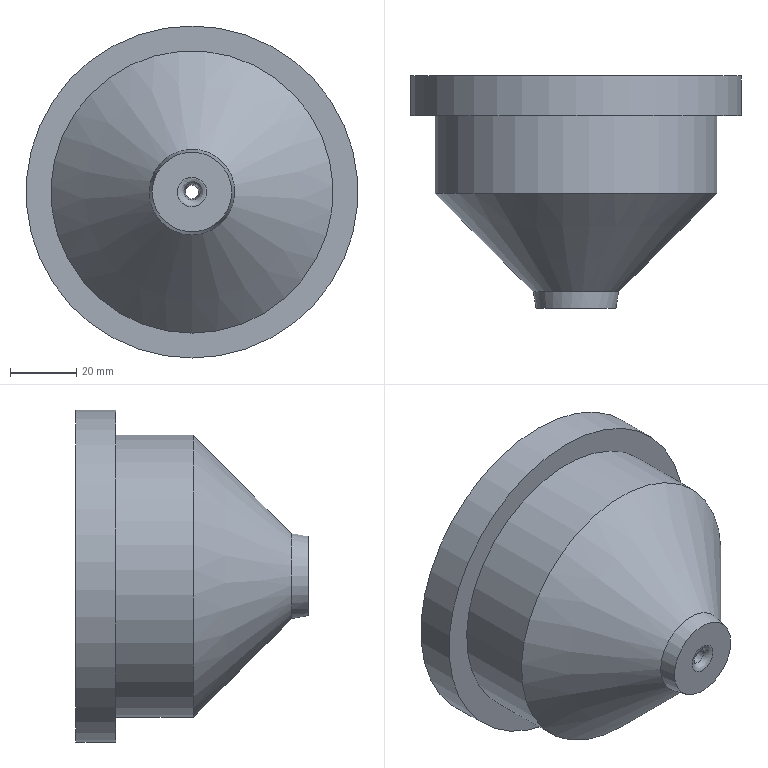Part | STEP file | SPRUE_id462_x_t | 1 solid | 13 faces | box 100 x 70 x 100 mm | volume 170232 mm3 | cone 4 | plane 3 | cylinder 3 | other 2 | spline 1 | commonest cylinder face diameters 65 x1 85 x1 100 x1
STEP:
#1=CARTESIAN_POINT('',(0.,90.5,-4.431));
#2=VERTEX_POINT('',#1);
#3=CARTESIAN_POINT('',(0.,90.5,4.431));
#4=VERTEX_POINT('',#3);
#5=CARTESIAN_POINT('',(0.,90.5,-4.431));
#6=CARTESIAN_POINT('',(0.2789,90.5,-4.431));
#7=CARTESIAN_POINT('',(0.5857,90.5,-4.396));
#8=CARTESIAN_POINT('',(0.906,90.5,-4.341));
#9=CARTESIAN_POINT('',(1.367,90.5,-4.225));
#10=CARTESIAN_POINT('',(1.776,90.5,-4.062));
#11=CARTESIAN_POINT('',(1.91,90.5,-4.001));
#12=CARTESIAN_POINT('',(2.106,90.5,-3.899));
#13=CARTESIAN_POINT('',(2.196,90.5,-3.848));
#14=CARTESIAN_POINT('',(2.22,90.5,-3.835));
#15=CARTESIAN_POINT('',(2.24,90.5,-3.823));
#16=CARTESIAN_POINT('',(2.373,90.5,-3.744));
#17=CARTESIAN_POINT('',(2.599,90.5,-3.611));
#18=CARTESIAN_POINT('',(3.199,90.5,-3.091));
#19=CARTESIAN_POINT('',(3.611,90.5,-2.603));
#20=CARTESIAN_POINT('',(4.042,90.5,-1.864));
#21=CARTESIAN_POINT('',(4.124,90.5,-1.623));
#22=CARTESIAN_POINT('',(4.164,90.5,-1.514));
#23=CARTESIAN_POINT('',(4.217,90.5,-1.369));
#24=CARTESIAN_POINT('',(4.294,90.5,-1.101));
#25=CARTESIAN_POINT('',(4.327,90.5,-0.9656));
#26=CARTESIAN_POINT('',(4.405,90.5,-0.5552));
#27=CARTESIAN_POINT('',(4.431,90.5,-0.2766));
#28=CARTESIAN_POINT('',(4.431,90.5,1.116));
#29=CARTESIAN_POINT('',(4.015,90.5,2.203));
#30=CARTESIAN_POINT('',(2.424,90.5,3.885));
#31=CARTESIAN_POINT('',(1.245,90.5,4.431));
#32=CARTESIAN_POINT('',(0.,90.5,4.431));
#33=B_SPLINE_CURVE_WITH_KNOTS('',3,(#5,#6,#7,#8,#9,#10,#11,#12,#13,#14,#15,#16,#17,#18,#19,#20,#21,#22,#23,#24,#25,#26,#27,#28,#29,#30,#31,#32),.UNSPECIFIED.,.F.,.F.,(4,2,2,2,2,2,2,2,2,2,2,2,2,4),(0.,0.0625,0.125,0.1562,0.1719,0.1875,0.25,0.3125,0.375,0.4062,0.4375,0.5,0.75,1.),.UNSPECIFIED.);
#34=EDGE_CURVE('',#2,#4,#33,.T.);
#35=ORIENTED_EDGE('',*,*,#34,.F.);
#36=CARTESIAN_POINT('',(0.,90.5,4.431));
#37=CARTESIAN_POINT('',(-8.862,90.5,4.431));
#38=CARTESIAN_POINT('',(-8.862,90.5,-4.431));
#39=CARTESIAN_POINT('',(0.,90.5,-4.431));
#40=(BOUNDED_CURVE()B_SPLINE_CURVE(3,(#36,#37,#38,#39),.UNSPECIFIED.,.F.,.F.)B_SPLINE_CURVE_WITH_KNOTS((4,4),(0.,1.),.UNSPECIFIED.)CURVE()GEOMETRIC_REPRESENTATION_ITEM()RATIONAL_B_SPLINE_CURVE((1.,0.3333,0.3333,1.))REPRESENTATION_ITEM(''));
#41=EDGE_CURVE('',#4,#2,#40,.T.);
#42=ORIENTED_EDGE('',*,*,#41,.F.);
#43=EDGE_LOOP('',(#35,#42));
#44=FACE_BOUND('',#43,.T.);
#45=CARTESIAN_POINT('',(-12.,90.5,0.));
#46=VERTEX_POINT('',#45);
#47=CARTESIAN_POINT('',(0.,90.5,0.));
#48=DIRECTION('',(0.,1.,0.));
#49=DIRECTION('',(-1.,0.,0.));
#50=AXIS2_PLACEMENT_3D('',#47,#48,#49);
#51=CIRCLE('',#50,12.);
#52=EDGE_CURVE('',#46,#46,#51,.T.);
#53=ORIENTED_EDGE('',*,*,#52,.F.);
#54=EDGE_LOOP('',(#53));
#55=FACE_BOUND('',#54,.T.);
#56=CARTESIAN_POINT('',(0.,90.5,0.));
#57=DIRECTION('',(0.,-1.,0.));
#58=DIRECTION('',(0.,0.,-1.));
#59=AXIS2_PLACEMENT_3D('',#56,#57,#58);
#60=PLANE('',#59);
#61=ADVANCED_FACE('',(#44,#55),#60,.T.);
#62=CARTESIAN_POINT('',(0.,92.43,2.432));
#63=VERTEX_POINT('',#62);
#64=CARTESIAN_POINT('',(0.,92.43,0.));
#65=DIRECTION('',(0.,1.,0.));
#66=DIRECTION('',(0.,0.,1.));
#67=AXIS2_PLACEMENT_3D('',#64,#65,#66);
#68=CIRCLE('',#67,2.432);
#69=EDGE_CURVE('',#63,#63,#68,.T.);
#70=ORIENTED_EDGE('',*,*,#69,.T.);
#71=EDGE_LOOP('',(#70));
#72=FACE_BOUND('',#71,.T.);
#73=ORIENTED_EDGE('',*,*,#41,.T.);
#74=ORIENTED_EDGE('',*,*,#34,.T.);
#75=EDGE_LOOP('',(#73,#74));
#76=FACE_BOUND('',#75,.T.);
#77=CARTESIAN_POINT('',(0.6761,92.5,-4.379));
#78=DIRECTION('',(0.9883,0.,0.1526));
#79=DIRECTION('',(0.1526,0.,-0.9883));
#80=AXIS2_PLACEMENT_3D('',#77,#78,#79);
#81=CIRCLE('',#80,2.);
#82=CARTESIAN_POINT('',(0.,92.5,0.));
#83=DIRECTION('',(0.,-1.,0.));
#84=AXIS1_PLACEMENT('',#82,#83);
#85=SURFACE_OF_REVOLUTION('',#81,#84);
#86=ADVANCED_FACE('',(#72,#76),#85,.F.);
#87=CARTESIAN_POINT('',(0.,95.5,-12.882));
#88=VERTEX_POINT('',#87);
#89=CARTESIAN_POINT('',(0.,95.5,0.));
#90=DIRECTION('',(0.,1.,0.));
#91=DIRECTION('',(0.,0.,-1.));
#92=AXIS2_PLACEMENT_3D('',#89,#90,#91);
#93=CIRCLE('',#92,12.882);
#94=EDGE_CURVE('',#88,#88,#93,.T.);
#95=ORIENTED_EDGE('',*,*,#94,.F.);
#96=EDGE_LOOP('',(#95));
#97=FACE_BOUND('',#96,.T.);
#98=ORIENTED_EDGE('',*,*,#52,.T.);
#99=EDGE_LOOP('',(#98));
#100=FACE_BOUND('',#99,.T.);
#101=CARTESIAN_POINT('',(0.,95.5,0.));
#102=DIRECTION('',(0.,1.,0.));
#103=DIRECTION('',(-1.,0.,0.));
#104=AXIS2_PLACEMENT_3D('',#101,#102,#103);
#105=CONICAL_SURFACE('',#104,12.882,10.);
#106=ADVANCED_FACE('',(#97,#100),#105,.T.);
#107=CARTESIAN_POINT('',(0.,104.736,-2.));
#108=VERTEX_POINT('',#107);
#109=CARTESIAN_POINT('',(0.,104.736,0.));
#110=DIRECTION('',(0.,1.,0.));
#111=DIRECTION('',(0.,0.,-1.));
#112=AXIS2_PLACEMENT_3D('',#109,#110,#111);
#113=CIRCLE('',#112,2.);
#114=EDGE_CURVE('',#108,#108,#113,.T.);
#115=ORIENTED_EDGE('',*,*,#114,.T.);
#116=EDGE_LOOP('',(#115));
#117=FACE_BOUND('',#116,.T.);
#118=ORIENTED_EDGE('',*,*,#69,.F.);
#119=EDGE_LOOP('',(#118));
#120=FACE_BOUND('',#119,.T.);
#121=CARTESIAN_POINT('',(0.,92.43,0.));
#122=DIRECTION('',(0.,-1.,0.));
#123=DIRECTION('',(0.,0.,-1.));
#124=AXIS2_PLACEMENT_3D('',#121,#122,#123);
#125=CONICAL_SURFACE('',#124,2.432,2.012);
#126=ADVANCED_FACE('',(#117,#120),#125,.F.);
#127=CARTESIAN_POINT('',(0.,125.118,-42.5));
#128=VERTEX_POINT('',#127);
#129=CARTESIAN_POINT('',(0.,125.118,0.));
#130=DIRECTION('',(0.,1.,0.));
#131=DIRECTION('',(0.,0.,-1.));
#132=AXIS2_PLACEMENT_3D('',#129,#130,#131);
#133=CIRCLE('',#132,42.5);
#134=EDGE_CURVE('',#128,#128,#133,.T.);
#135=ORIENTED_EDGE('',*,*,#134,.F.);
#136=EDGE_LOOP('',(#135));
#137=FACE_BOUND('',#136,.T.);
#138=ORIENTED_EDGE('',*,*,#94,.T.);
#139=EDGE_LOOP('',(#138));
#140=FACE_BOUND('',#139,.T.);
#141=CARTESIAN_POINT('',(0.,125.118,0.));
#142=DIRECTION('',(0.,1.,0.));
#143=DIRECTION('',(0.,0.,1.));
#144=AXIS2_PLACEMENT_3D('',#141,#142,#143);
#145=CONICAL_SURFACE('',#144,42.5,45.);
#146=ADVANCED_FACE('',(#137,#140),#145,.T.);
#147=ORIENTED_EDGE('',*,*,#114,.F.);
#148=EDGE_LOOP('',(#147));
#149=FACE_BOUND('',#148,.T.);
#150=CARTESIAN_POINT('',(-13.435,110.196,0.));
#151=VERTEX_POINT('',#150);
#152=CARTESIAN_POINT('',(0.,110.196,0.));
#153=DIRECTION('',(0.,1.,0.));
#154=DIRECTION('',(-1.,0.,0.));
#155=AXIS2_PLACEMENT_3D('',#152,#153,#154);
#156=CIRCLE('',#155,13.435);
#157=EDGE_CURVE('',#151,#151,#156,.T.);
#158=ORIENTED_EDGE('',*,*,#157,.T.);
#159=EDGE_LOOP('',(#158));
#160=FACE_BOUND('',#159,.T.);
#161=CARTESIAN_POINT('',(-13.26,123.631,13.608));
#162=CARTESIAN_POINT('',(-21.423,123.631,5.653));
#163=CARTESIAN_POINT('',(-21.399,123.631,-5.745));
#164=CARTESIAN_POINT('',(-13.202,123.631,-13.664));
#165=(BOUNDED_CURVE()B_SPLINE_CURVE(3,(#161,#162,#163,#164),.UNSPECIFIED.,.F.,.F.)B_SPLINE_CURVE_WITH_KNOTS((4,4),(0.,1.),.UNSPECIFIED.)CURVE()GEOMETRIC_REPRESENTATION_ITEM()RATIONAL_B_SPLINE_CURVE((1.,0.7976,0.7976,1.))REPRESENTATION_ITEM(''));
#166=CARTESIAN_POINT('',(0.,123.631,0.));
#167=DIRECTION('',(0.,0.,1.));
#168=AXIS1_PLACEMENT('',#166,#167);
#169=SURFACE_OF_REVOLUTION('',#165,#168);
#170=ADVANCED_FACE('',(#149,#160),#169,.T.);
#171=CARTESIAN_POINT('',(0.,148.5,-42.5));
#172=VERTEX_POINT('',#171);
#173=CARTESIAN_POINT('',(0.,148.5,0.));
#174=DIRECTION('',(0.,1.,0.));
#175=DIRECTION('',(0.,0.,-1.));
#176=AXIS2_PLACEMENT_3D('',#173,#174,#175);
#177=CIRCLE('',#176,42.5);
#178=EDGE_CURVE('',#172,#172,#177,.T.);
#179=ORIENTED_EDGE('',*,*,#178,.F.);
#180=EDGE_LOOP('',(#179));
#181=FACE_BOUND('',#180,.T.);
#182=ORIENTED_EDGE('',*,*,#134,.T.);
#183=EDGE_LOOP('',(#182));
#184=FACE_BOUND('',#183,.T.);
#185=CARTESIAN_POINT('',(0.,164.,0.));
#186=DIRECTION('',(0.,-1.,0.));
#187=DIRECTION('',(0.,0.,-1.));
#188=AXIS2_PLACEMENT_3D('',#185,#186,#187);
#189=CYLINDRICAL_SURFACE('',#188,42.5);
#190=ADVANCED_FACE('',(#181,#184),#189,.T.);
#191=ORIENTED_EDGE('',*,*,#157,.F.);
#192=EDGE_LOOP('',(#191));
#193=FACE_BOUND('',#192,.T.);
#194=CARTESIAN_POINT('',(0.,123.403,26.642));
#195=VERTEX_POINT('',#194);
#196=CARTESIAN_POINT('',(0.,123.403,0.));
#197=DIRECTION('',(0.,1.,0.));
#198=DIRECTION('',(0.,0.,1.));
#199=AXIS2_PLACEMENT_3D('',#196,#197,#198);
#200=CIRCLE('',#199,26.642);
#201=EDGE_CURVE('',#195,#195,#200,.T.);
#202=ORIENTED_EDGE('',*,*,#201,.T.);
#203=EDGE_LOOP('',(#202));
#204=FACE_BOUND('',#203,.T.);
#205=CARTESIAN_POINT('',(0.,123.403,0.));
#206=DIRECTION('',(0.,1.,0.));
#207=DIRECTION('',(-1.,0.,0.));
#208=AXIS2_PLACEMENT_3D('',#205,#206,#207);
#209=CONICAL_SURFACE('',#208,26.642,45.);
#210=ADVANCED_FACE('',(#193,#204),#209,.F.);
#211=ORIENTED_EDGE('',*,*,#178,.T.);
#212=EDGE_LOOP('',(#211));
#213=FACE_BOUND('',#212,.T.);
#214=CARTESIAN_POINT('',(0.,148.5,-50.));
#215=VERTEX_POINT('',#214);
#216=CARTESIAN_POINT('',(0.,148.5,0.));
#217=DIRECTION('',(0.,1.,0.));
#218=DIRECTION('',(0.,0.,-1.));
#219=AXIS2_PLACEMENT_3D('',#216,#217,#218);
#220=CIRCLE('',#219,50.);
#221=EDGE_CURVE('',#215,#215,#220,.T.);
#222=ORIENTED_EDGE('',*,*,#221,.F.);
#223=EDGE_LOOP('',(#222));
#224=FACE_BOUND('',#223,.T.);
#225=CARTESIAN_POINT('',(0.,148.5,0.));
#226=DIRECTION('',(0.,-1.,0.));
#227=DIRECTION('',(0.,0.,-1.));
#228=AXIS2_PLACEMENT_3D('',#225,#226,#227);
#229=PLANE('',#228);
#230=ADVANCED_FACE('',(#213,#224),#229,.T.);
#231=ORIENTED_EDGE('',*,*,#201,.F.);
#232=EDGE_LOOP('',(#231));
#233=FACE_BOUND('',#232,.T.);
#234=CARTESIAN_POINT('',(0.,137.545,-32.5));
#235=VERTEX_POINT('',#234);
#236=CARTESIAN_POINT('',(0.,137.545,0.));
#237=DIRECTION('',(0.,1.,0.));
#238=DIRECTION('',(0.,0.,-1.));
#239=AXIS2_PLACEMENT_3D('',#236,#237,#238);
#240=CIRCLE('',#239,32.5);
#241=EDGE_CURVE('',#235,#235,#240,.T.);
#242=ORIENTED_EDGE('',*,*,#241,.T.);
#243=EDGE_LOOP('',(#242));
#244=FACE_BOUND('',#243,.T.);
#245=CARTESIAN_POINT('',(0.,137.545,-32.5));
#246=CARTESIAN_POINT('',(65.,137.545,-32.5));
#247=CARTESIAN_POINT('',(65.,137.545,32.5));
#248=CARTESIAN_POINT('',(0.,137.545,32.5));
#249=CARTESIAN_POINT('',(-65.,137.545,32.5));
#250=CARTESIAN_POINT('',(-65.,137.545,-32.5));
#251=CARTESIAN_POINT('',(0.,137.545,-32.5));
#252=CARTESIAN_POINT('',(0.,132.17,-32.5));
#253=CARTESIAN_POINT('',(65.,132.17,-32.5));
#254=CARTESIAN_POINT('',(65.,132.17,32.5));
#255=CARTESIAN_POINT('',(0.,132.17,32.5));
#256=CARTESIAN_POINT('',(-65.,132.17,32.5));
#257=CARTESIAN_POINT('',(-65.,132.17,-32.5));
#258=CARTESIAN_POINT('',(0.,132.17,-32.5));
#259=CARTESIAN_POINT('',(0.,127.203,-30.443));
#260=CARTESIAN_POINT('',(60.886,127.203,-30.443));
#261=CARTESIAN_POINT('',(60.886,127.203,30.443));
#262=CARTESIAN_POINT('',(0.,127.203,30.443));
#263=CARTESIAN_POINT('',(-60.886,127.203,30.443));
#264=CARTESIAN_POINT('',(-60.886,127.203,-30.443));
#265=CARTESIAN_POINT('',(0.,127.203,-30.443));
#266=CARTESIAN_POINT('',(0.,123.403,-26.642));
#267=CARTESIAN_POINT('',(53.284,123.403,-26.642));
#268=CARTESIAN_POINT('',(53.284,123.403,26.642));
#269=CARTESIAN_POINT('',(0.,123.403,26.642));
#270=CARTESIAN_POINT('',(-53.284,123.403,26.642));
#271=CARTESIAN_POINT('',(-53.284,123.403,-26.642));
#272=CARTESIAN_POINT('',(0.,123.403,-26.642));
#273=(BOUNDED_SURFACE()B_SPLINE_SURFACE(3,3,((#245,#246,#247,#248,#249,#250,#251),(#252,#253,#254,#255,#256,#257,#258),(#259,#260,#261,#262,#263,#264,#265),(#266,#267,#268,#269,#270,#271,#272)),.UNSPECIFIED.,.F.,.T.,.F.)B_SPLINE_SURFACE_WITH_KNOTS((4,4),(1,3,3,3,1),(0.,1.),(-0.5,0.,0.5,1.,1.5),.UNSPECIFIED.)GEOMETRIC_REPRESENTATION_ITEM()RATIONAL_B_SPLINE_SURFACE(((1.,0.3333,0.3333,1.,0.3333,0.3333,1.),(0.9493,0.3164,0.3164,0.9493,0.3164,0.3164,0.9493),(0.9493,0.3164,0.3164,0.9493,0.3164,0.3164,0.9493),(1.,0.3333,0.3333,1.,0.3333,0.3333,1.)))REPRESENTATION_ITEM('')SURFACE());
#274=ADVANCED_FACE('',(#233,#244),#273,.T.);
#275=ORIENTED_EDGE('',*,*,#221,.T.);
#276=EDGE_LOOP('',(#275));
#277=FACE_BOUND('',#276,.T.);
#278=CARTESIAN_POINT('',(0.,160.5,-50.));
#279=VERTEX_POINT('',#278);
#280=CARTESIAN_POINT('',(0.,160.5,0.));
#281=DIRECTION('',(0.,-1.,0.));
#282=DIRECTION('',(0.,0.,-1.));
#283=AXIS2_PLACEMENT_3D('',#280,#281,#282);
#284=CIRCLE('',#283,50.);
#285=EDGE_CURVE('',#279,#279,#284,.T.);
#286=ORIENTED_EDGE('',*,*,#285,.T.);
#287=EDGE_LOOP('',(#286));
#288=FACE_BOUND('',#287,.T.);
#289=CARTESIAN_POINT('',(0.,164.,0.));
#290=DIRECTION('',(0.,-1.,0.));
#291=DIRECTION('',(0.,0.,-1.));
#292=AXIS2_PLACEMENT_3D('',#289,#290,#291);
#293=CYLINDRICAL_SURFACE('',#292,50.);
#294=ADVANCED_FACE('',(#277,#288),#293,.T.);
#295=ORIENTED_EDGE('',*,*,#241,.F.);
#296=EDGE_LOOP('',(#295));
#297=FACE_BOUND('',#296,.T.);
#298=CARTESIAN_POINT('',(0.,160.5,-32.5));
#299=VERTEX_POINT('',#298);
#300=CARTESIAN_POINT('',(0.,160.5,0.));
#301=DIRECTION('',(0.,1.,0.));
#302=DIRECTION('',(0.,0.,-1.));
#303=AXIS2_PLACEMENT_3D('',#300,#301,#302);
#304=CIRCLE('',#303,32.5);
#305=EDGE_CURVE('',#299,#299,#304,.T.);
#306=ORIENTED_EDGE('',*,*,#305,.T.);
#307=EDGE_LOOP('',(#306));
#308=FACE_BOUND('',#307,.T.);
#309=CARTESIAN_POINT('',(0.,164.,0.));
#310=DIRECTION('',(0.,-1.,0.));
#311=DIRECTION('',(0.,0.,-1.));
#312=AXIS2_PLACEMENT_3D('',#309,#310,#311);
#313=CYLINDRICAL_SURFACE('',#312,32.5);
#314=ADVANCED_FACE('',(#297,#308),#313,.F.);
#315=ORIENTED_EDGE('',*,*,#305,.F.);
#316=EDGE_LOOP('',(#315));
#317=FACE_BOUND('',#316,.T.);
#318=ORIENTED_EDGE('',*,*,#285,.F.);
#319=EDGE_LOOP('',(#318));
#320=FACE_BOUND('',#319,.T.);
#321=CARTESIAN_POINT('',(0.,160.5,0.));
#322=DIRECTION('',(0.,-1.,0.));
#323=DIRECTION('',(0.,0.,-1.));
#324=AXIS2_PLACEMENT_3D('',#321,#322,#323);
#325=PLANE('',#324);
#326=ADVANCED_FACE('',(#317,#320),#325,.F.);
#327=CLOSED_SHELL('',(#61,#86,#106,#126,#146,#170,#190,#210,#230,#274,#294,#314,#326));
#328=MANIFOLD_SOLID_BREP('',#327);
#329=(LENGTH_UNIT()NAMED_UNIT(*)SI_UNIT(.MILLI.,.METRE.));
#330=UNCERTAINTY_MEASURE_WITH_UNIT(LENGTH_MEASURE(0.0508),#329,'','');
#331=(NAMED_UNIT(*)PLANE_ANGLE_UNIT()SI_UNIT($,.RADIAN.));
#332=PLANE_ANGLE_MEASURE_WITH_UNIT(PLANE_ANGLE_MEASURE(0.01745),#331);
#333=DIMENSIONAL_EXPONENTS(0.,0.,0.,0.,0.,0.,0.);
#334=(CONVERSION_BASED_UNIT('DEGREE',#332)NAMED_UNIT(#333)PLANE_ANGLE_UNIT());
#335=(NAMED_UNIT(*)SI_UNIT($,.STERADIAN.)SOLID_ANGLE_UNIT());
#336=(GEOMETRIC_REPRESENTATION_CONTEXT(3)GLOBAL_UNCERTAINTY_ASSIGNED_CONTEXT((#330))GLOBAL_UNIT_ASSIGNED_CONTEXT((#329,#334,#335))REPRESENTATION_CONTEXT('',''));
#337=ADVANCED_BREP_SHAPE_REPRESENTATION('',(#328),#336);